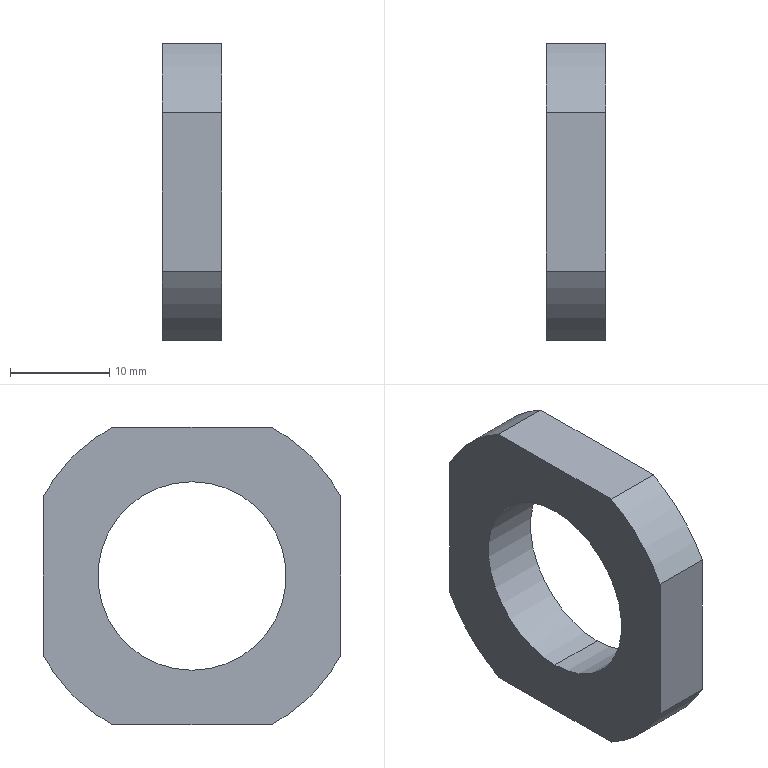Part | STEP file | PN_0005 nut | 1 solid | 12 faces | box 6 x 30 x 30 mm | volume 3228 mm3 | cylinder 6 | plane 6 | commonest cylinder face diameters 34 x4 19 x2
STEP:
#1=CARTESIAN_POINT('',(0.,0.,0.));
#2=DIRECTION('',(0.,0.,1.));
#3=DIRECTION('',(1.,0.,0.));
#4=AXIS2_PLACEMENT_3D('',#1,#2,#3);
#5=CARTESIAN_POINT('',(0.,0.,9.5));
#6=VERTEX_POINT('',#5);
#7=CARTESIAN_POINT('',(-6.,0.,9.5));
#8=VERTEX_POINT('',#7);
#9=CARTESIAN_POINT('',(0.,0.,9.5));
#10=DIRECTION('',(-1.,0.,0.));
#11=VECTOR('',#10,1.);
#12=LINE('',#9,#11);
#13=CARTESIAN_POINT('',(0.,0.,0.));
#14=DIRECTION('',(-1.,0.,0.));
#15=DIRECTION('',(0.,0.,1.));
#16=AXIS2_PLACEMENT_3D('',#13,#14,#15);
#17=CYLINDRICAL_SURFACE('',#16,9.5);
#18=CARTESIAN_POINT('',(6.283,0.));
#19=DIRECTION('',(0.,1.));
#20=VECTOR('',#19,1.);
#21=LINE('',#18,#20);
#22=(GEOMETRIC_REPRESENTATION_CONTEXT(2)PARAMETRIC_REPRESENTATION_CONTEXT()REPRESENTATION_CONTEXT('',''));
#23=DEFINITIONAL_REPRESENTATION('',(#21),#22);
#24=PCURVE('',#17,#23);
#25=CARTESIAN_POINT('',(0.,0.,0.));
#26=DIRECTION('',(-1.,0.,0.));
#27=DIRECTION('',(0.,0.,1.));
#28=AXIS2_PLACEMENT_3D('',#25,#26,#27);
#29=CYLINDRICAL_SURFACE('',#28,9.5);
#30=CARTESIAN_POINT('',(0.,0.));
#31=DIRECTION('',(0.,1.));
#32=VECTOR('',#31,1.);
#33=LINE('',#30,#32);
#34=(GEOMETRIC_REPRESENTATION_CONTEXT(2)PARAMETRIC_REPRESENTATION_CONTEXT()REPRESENTATION_CONTEXT('',''));
#35=DEFINITIONAL_REPRESENTATION('',(#33),#34);
#36=PCURVE('',#29,#35);
#37=SURFACE_CURVE('',#12,(#24,#36),.PCURVE_S1.);
#38=EDGE_CURVE('',#6,#8,#37,.T.);
#39=ORIENTED_EDGE('',*,*,#38,.T.);
#40=CARTESIAN_POINT('',(-6.,0.,-9.5));
#41=VERTEX_POINT('',#40);
#42=CARTESIAN_POINT('',(-6.,0.,0.));
#43=DIRECTION('',(1.,0.,0.));
#44=DIRECTION('',(0.,0.,-1.));
#45=AXIS2_PLACEMENT_3D('',#42,#43,#44);
#46=CIRCLE('',#45,9.5);
#47=CARTESIAN_POINT('',(9.425,6.));
#48=DIRECTION('',(-1.,0.));
#49=VECTOR('',#48,1.);
#50=LINE('',#47,#49);
#51=(GEOMETRIC_REPRESENTATION_CONTEXT(2)PARAMETRIC_REPRESENTATION_CONTEXT()REPRESENTATION_CONTEXT('',''));
#52=DEFINITIONAL_REPRESENTATION('',(#50),#51);
#53=PCURVE('',#17,#52);
#54=CARTESIAN_POINT('',(-6.,17.,0.));
#55=DIRECTION('',(-1.,0.,0.));
#56=DIRECTION('',(0.,0.,1.));
#57=AXIS2_PLACEMENT_3D('',#54,#55,#56);
#58=PLANE('',#57);
#59=CARTESIAN_POINT('',(-9.5,-17.));
#60=CARTESIAN_POINT('',(-9.5,-0.5455));
#61=CARTESIAN_POINT('',(4.75,-8.773));
#62=CARTESIAN_POINT('',(19.,-17.));
#63=CARTESIAN_POINT('',(4.75,-25.227));
#64=CARTESIAN_POINT('',(-9.5,-33.454));
#65=CARTESIAN_POINT('',(-9.5,-17.));
#66=(BOUNDED_CURVE()B_SPLINE_CURVE(2,(#59,#60,#61,#62,#63,#64,#65),.UNSPECIFIED.,.T.,.F.)B_SPLINE_CURVE_WITH_KNOTS((1,2,2,2,2,1),(-2.094,0.,2.094,4.189,6.283,8.378),.UNSPECIFIED.)CURVE()GEOMETRIC_REPRESENTATION_ITEM()RATIONAL_B_SPLINE_CURVE((1.,0.5,1.,0.5,1.,0.5,1.))REPRESENTATION_ITEM(''));
#67=(GEOMETRIC_REPRESENTATION_CONTEXT(2)PARAMETRIC_REPRESENTATION_CONTEXT()REPRESENTATION_CONTEXT('',''));
#68=DEFINITIONAL_REPRESENTATION('',(#66),#67);
#69=PCURVE('',#58,#68);
#70=SURFACE_CURVE('',#46,(#53,#69),.PCURVE_S1.);
#71=EDGE_CURVE('',#8,#41,#70,.T.);
#72=ORIENTED_EDGE('',*,*,#71,.T.);
#73=CARTESIAN_POINT('',(0.,0.,-9.5));
#74=VERTEX_POINT('',#73);
#75=CARTESIAN_POINT('',(0.,0.,-9.5));
#76=DIRECTION('',(-1.,0.,0.));
#77=VECTOR('',#76,1.);
#78=LINE('',#75,#77);
#79=CARTESIAN_POINT('',(3.142,0.));
#80=DIRECTION('',(0.,1.));
#81=VECTOR('',#80,1.);
#82=LINE('',#79,#81);
#83=(GEOMETRIC_REPRESENTATION_CONTEXT(2)PARAMETRIC_REPRESENTATION_CONTEXT()REPRESENTATION_CONTEXT('',''));
#84=DEFINITIONAL_REPRESENTATION('',(#82),#83);
#85=PCURVE('',#17,#84);
#86=CARTESIAN_POINT('',(3.142,0.));
#87=DIRECTION('',(0.,1.));
#88=VECTOR('',#87,1.);
#89=LINE('',#86,#88);
#90=(GEOMETRIC_REPRESENTATION_CONTEXT(2)PARAMETRIC_REPRESENTATION_CONTEXT()REPRESENTATION_CONTEXT('',''));
#91=DEFINITIONAL_REPRESENTATION('',(#89),#90);
#92=PCURVE('',#29,#91);
#93=SURFACE_CURVE('',#78,(#85,#92),.PCURVE_S1.);
#94=EDGE_CURVE('',#74,#41,#93,.T.);
#95=ORIENTED_EDGE('',*,*,#94,.F.);
#96=CARTESIAN_POINT('',(0.,0.,0.));
#97=DIRECTION('',(1.,0.,0.));
#98=DIRECTION('',(0.,0.,-1.));
#99=AXIS2_PLACEMENT_3D('',#96,#97,#98);
#100=CIRCLE('',#99,9.5);
#101=CARTESIAN_POINT('',(9.425,0.));
#102=DIRECTION('',(-1.,0.));
#103=VECTOR('',#102,1.);
#104=LINE('',#101,#103);
#105=(GEOMETRIC_REPRESENTATION_CONTEXT(2)PARAMETRIC_REPRESENTATION_CONTEXT()REPRESENTATION_CONTEXT('',''));
#106=DEFINITIONAL_REPRESENTATION('',(#104),#105);
#107=PCURVE('',#17,#106);
#108=CARTESIAN_POINT('',(0.,0.,0.));
#109=DIRECTION('',(1.,0.,0.));
#110=DIRECTION('',(0.,0.,-1.));
#111=AXIS2_PLACEMENT_3D('',#108,#109,#110);
#112=PLANE('',#111);
#113=CARTESIAN_POINT('',(0.,0.));
#114=DIRECTION('',(1.,0.));
#115=AXIS2_PLACEMENT_2D('',#113,#114);
#116=CIRCLE('',#115,9.5);
#117=(GEOMETRIC_REPRESENTATION_CONTEXT(2)PARAMETRIC_REPRESENTATION_CONTEXT()REPRESENTATION_CONTEXT('',''));
#118=DEFINITIONAL_REPRESENTATION('',(#116),#117);
#119=PCURVE('',#112,#118);
#120=SURFACE_CURVE('',#100,(#107,#119),.PCURVE_S1.);
#121=EDGE_CURVE('',#6,#74,#120,.T.);
#122=ORIENTED_EDGE('',*,*,#121,.F.);
#123=EDGE_LOOP('',(#39,#72,#95,#122));
#124=FACE_BOUND('',#123,.F.);
#125=ADVANCED_FACE('',(#124),#17,.F.);
#126=CARTESIAN_POINT('',(0.,8.,15.));
#127=VERTEX_POINT('',#126);
#128=CARTESIAN_POINT('',(-6.,8.,15.));
#129=VERTEX_POINT('',#128);
#130=CARTESIAN_POINT('',(0.,8.,15.));
#131=DIRECTION('',(-1.,0.,0.));
#132=VECTOR('',#131,1.);
#133=LINE('',#130,#132);
#134=CARTESIAN_POINT('',(0.,0.,0.));
#135=DIRECTION('',(1.,0.,0.));
#136=DIRECTION('',(0.,0.,-1.));
#137=AXIS2_PLACEMENT_3D('',#134,#135,#136);
#138=CYLINDRICAL_SURFACE('',#137,17.);
#139=CARTESIAN_POINT('',(2.652,0.));
#140=DIRECTION('',(0.,-1.));
#141=VECTOR('',#140,1.);
#142=LINE('',#139,#141);
#143=(GEOMETRIC_REPRESENTATION_CONTEXT(2)PARAMETRIC_REPRESENTATION_CONTEXT()REPRESENTATION_CONTEXT('',''));
#144=DEFINITIONAL_REPRESENTATION('',(#142),#143);
#145=PCURVE('',#138,#144);
#146=CARTESIAN_POINT('',(0.,17.205,15.));
#147=DIRECTION('',(0.,0.,-1.));
#148=DIRECTION('',(0.,1.,0.));
#149=AXIS2_PLACEMENT_3D('',#146,#147,#148);
#150=PLANE('',#149);
#151=CARTESIAN_POINT('',(-9.205,0.));
#152=DIRECTION('',(0.,-1.));
#153=VECTOR('',#152,1.);
#154=LINE('',#151,#153);
#155=(GEOMETRIC_REPRESENTATION_CONTEXT(2)PARAMETRIC_REPRESENTATION_CONTEXT()REPRESENTATION_CONTEXT('',''));
#156=DEFINITIONAL_REPRESENTATION('',(#154),#155);
#157=PCURVE('',#150,#156);
#158=SURFACE_CURVE('',#133,(#145,#157),.PCURVE_S1.);
#159=EDGE_CURVE('',#127,#129,#158,.T.);
#160=ORIENTED_EDGE('',*,*,#159,.F.);
#161=CARTESIAN_POINT('',(0.,15.,8.));
#162=VERTEX_POINT('',#161);
#163=CARTESIAN_POINT('',(0.,0.,0.));
#164=DIRECTION('',(1.,0.,0.));
#165=DIRECTION('',(0.,0.,-1.));
#166=AXIS2_PLACEMENT_3D('',#163,#164,#165);
#167=CIRCLE('',#166,17.);
#168=CARTESIAN_POINT('',(0.,0.));
#169=DIRECTION('',(1.,0.));
#170=VECTOR('',#169,1.);
#171=LINE('',#168,#170);
#172=(GEOMETRIC_REPRESENTATION_CONTEXT(2)PARAMETRIC_REPRESENTATION_CONTEXT()REPRESENTATION_CONTEXT('',''));
#173=DEFINITIONAL_REPRESENTATION('',(#171),#172);
#174=PCURVE('',#138,#173);
#175=CARTESIAN_POINT('',(0.,0.));
#176=DIRECTION('',(1.,0.));
#177=AXIS2_PLACEMENT_2D('',#175,#176);
#178=CIRCLE('',#177,17.);
#179=(GEOMETRIC_REPRESENTATION_CONTEXT(2)PARAMETRIC_REPRESENTATION_CONTEXT()REPRESENTATION_CONTEXT('',''));
#180=DEFINITIONAL_REPRESENTATION('',(#178),#179);
#181=PCURVE('',#112,#180);
#182=SURFACE_CURVE('',#167,(#174,#181),.PCURVE_S1.);
#183=EDGE_CURVE('',#162,#127,#182,.T.);
#184=ORIENTED_EDGE('',*,*,#183,.F.);
#185=CARTESIAN_POINT('',(-6.,15.,8.));
#186=VERTEX_POINT('',#185);
#187=CARTESIAN_POINT('',(0.,15.,8.));
#188=DIRECTION('',(1.,0.,0.));
#189=VECTOR('',#188,1.);
#190=LINE('',#187,#189);
#191=CARTESIAN_POINT('',(2.061,0.));
#192=DIRECTION('',(0.,1.));
#193=VECTOR('',#192,1.);
#194=LINE('',#191,#193);
#195=(GEOMETRIC_REPRESENTATION_CONTEXT(2)PARAMETRIC_REPRESENTATION_CONTEXT()REPRESENTATION_CONTEXT('',''));
#196=DEFINITIONAL_REPRESENTATION('',(#194),#195);
#197=PCURVE('',#138,#196);
#198=CARTESIAN_POINT('',(0.,15.,-20.296));
#199=DIRECTION('',(0.,-1.,0.));
#200=DIRECTION('',(0.,0.,-1.));
#201=AXIS2_PLACEMENT_3D('',#198,#199,#200);
#202=PLANE('',#201);
#203=CARTESIAN_POINT('',(-28.296,0.));
#204=DIRECTION('',(0.,1.));
#205=VECTOR('',#204,1.);
#206=LINE('',#203,#205);
#207=(GEOMETRIC_REPRESENTATION_CONTEXT(2)PARAMETRIC_REPRESENTATION_CONTEXT()REPRESENTATION_CONTEXT('',''));
#208=DEFINITIONAL_REPRESENTATION('',(#206),#207);
#209=PCURVE('',#202,#208);
#210=SURFACE_CURVE('',#190,(#197,#209),.PCURVE_S1.);
#211=EDGE_CURVE('',#186,#162,#210,.T.);
#212=ORIENTED_EDGE('',*,*,#211,.F.);
#213=CARTESIAN_POINT('',(-6.,0.,0.));
#214=DIRECTION('',(1.,0.,0.));
#215=DIRECTION('',(0.,0.,-1.));
#216=AXIS2_PLACEMENT_3D('',#213,#214,#215);
#217=CIRCLE('',#216,17.);
#218=CARTESIAN_POINT('',(0.,-6.));
#219=DIRECTION('',(1.,0.));
#220=VECTOR('',#219,1.);
#221=LINE('',#218,#220);
#222=(GEOMETRIC_REPRESENTATION_CONTEXT(2)PARAMETRIC_REPRESENTATION_CONTEXT()REPRESENTATION_CONTEXT('',''));
#223=DEFINITIONAL_REPRESENTATION('',(#221),#222);
#224=PCURVE('',#138,#223);
#225=CARTESIAN_POINT('',(-17.,-17.));
#226=CARTESIAN_POINT('',(-17.,12.445));
#227=CARTESIAN_POINT('',(8.5,-2.278));
#228=CARTESIAN_POINT('',(34.,-17.));
#229=CARTESIAN_POINT('',(8.5,-31.722));
#230=CARTESIAN_POINT('',(-17.,-46.445));
#231=CARTESIAN_POINT('',(-17.,-17.));
#232=(BOUNDED_CURVE()B_SPLINE_CURVE(2,(#225,#226,#227,#228,#229,#230,#231),.UNSPECIFIED.,.T.,.F.)B_SPLINE_CURVE_WITH_KNOTS((1,2,2,2,2,1),(-2.094,0.,2.094,4.189,6.283,8.378),.UNSPECIFIED.)CURVE()GEOMETRIC_REPRESENTATION_ITEM()RATIONAL_B_SPLINE_CURVE((1.,0.5,1.,0.5,1.,0.5,1.))REPRESENTATION_ITEM(''));
#233=(GEOMETRIC_REPRESENTATION_CONTEXT(2)PARAMETRIC_REPRESENTATION_CONTEXT()REPRESENTATION_CONTEXT('',''));
#234=DEFINITIONAL_REPRESENTATION('',(#232),#233);
#235=PCURVE('',#58,#234);
#236=SURFACE_CURVE('',#217,(#224,#235),.PCURVE_S1.);
#237=EDGE_CURVE('',#186,#129,#236,.T.);
#238=ORIENTED_EDGE('',*,*,#237,.T.);
#239=EDGE_LOOP('',(#160,#184,#212,#238));
#240=FACE_BOUND('',#239,.T.);
#241=ADVANCED_FACE('',(#240),#138,.T.);
#242=CARTESIAN_POINT('',(0.,-8.,-15.));
#243=VERTEX_POINT('',#242);
#244=CARTESIAN_POINT('',(-6.,-8.,-15.));
#245=VERTEX_POINT('',#244);
#246=CARTESIAN_POINT('',(0.,-8.,-15.));
#247=DIRECTION('',(-1.,0.,0.));
#248=VECTOR('',#247,1.);
#249=LINE('',#246,#248);
#250=CARTESIAN_POINT('',(0.,0.,0.));
#251=DIRECTION('',(1.,0.,0.));
#252=DIRECTION('',(0.,0.,-1.));
#253=AXIS2_PLACEMENT_3D('',#250,#251,#252);
#254=CYLINDRICAL_SURFACE('',#253,17.);
#255=CARTESIAN_POINT('',(5.793,0.));
#256=DIRECTION('',(0.,-1.));
#257=VECTOR('',#256,1.);
#258=LINE('',#255,#257);
#259=(GEOMETRIC_REPRESENTATION_CONTEXT(2)PARAMETRIC_REPRESENTATION_CONTEXT()REPRESENTATION_CONTEXT('',''));
#260=DEFINITIONAL_REPRESENTATION('',(#258),#259);
#261=PCURVE('',#254,#260);
#262=CARTESIAN_POINT('',(0.,17.205,-15.));
#263=DIRECTION('',(0.,0.,1.));
#264=DIRECTION('',(0.,-1.,0.));
#265=AXIS2_PLACEMENT_3D('',#262,#263,#264);
#266=PLANE('',#265);
#267=CARTESIAN_POINT('',(25.205,0.));
#268=DIRECTION('',(0.,-1.));
#269=VECTOR('',#268,1.);
#270=LINE('',#267,#269);
#271=(GEOMETRIC_REPRESENTATION_CONTEXT(2)PARAMETRIC_REPRESENTATION_CONTEXT()REPRESENTATION_CONTEXT('',''));
#272=DEFINITIONAL_REPRESENTATION('',(#270),#271);
#273=PCURVE('',#266,#272);
#274=SURFACE_CURVE('',#249,(#261,#273),.PCURVE_S1.);
#275=EDGE_CURVE('',#243,#245,#274,.T.);
#276=ORIENTED_EDGE('',*,*,#275,.F.);
#277=CARTESIAN_POINT('',(0.,-15.,-8.));
#278=VERTEX_POINT('',#277);
#279=CARTESIAN_POINT('',(0.,0.,0.));
#280=DIRECTION('',(1.,0.,0.));
#281=DIRECTION('',(0.,0.,-1.));
#282=AXIS2_PLACEMENT_3D('',#279,#280,#281);
#283=CIRCLE('',#282,17.);
#284=CARTESIAN_POINT('',(0.,0.));
#285=DIRECTION('',(1.,0.));
#286=VECTOR('',#285,1.);
#287=LINE('',#284,#286);
#288=(GEOMETRIC_REPRESENTATION_CONTEXT(2)PARAMETRIC_REPRESENTATION_CONTEXT()REPRESENTATION_CONTEXT('',''));
#289=DEFINITIONAL_REPRESENTATION('',(#287),#288);
#290=PCURVE('',#254,#289);
#291=CARTESIAN_POINT('',(0.,0.));
#292=DIRECTION('',(1.,0.));
#293=AXIS2_PLACEMENT_2D('',#291,#292);
#294=CIRCLE('',#293,17.);
#295=(GEOMETRIC_REPRESENTATION_CONTEXT(2)PARAMETRIC_REPRESENTATION_CONTEXT()REPRESENTATION_CONTEXT('',''));
#296=DEFINITIONAL_REPRESENTATION('',(#294),#295);
#297=PCURVE('',#112,#296);
#298=SURFACE_CURVE('',#283,(#290,#297),.PCURVE_S1.);
#299=EDGE_CURVE('',#278,#243,#298,.T.);
#300=ORIENTED_EDGE('',*,*,#299,.F.);
#301=CARTESIAN_POINT('',(-6.,-15.,-8.));
#302=VERTEX_POINT('',#301);
#303=CARTESIAN_POINT('',(0.,-15.,-8.));
#304=DIRECTION('',(1.,0.,0.));
#305=VECTOR('',#304,1.);
#306=LINE('',#303,#305);
#307=CARTESIAN_POINT('',(5.202,0.));
#308=DIRECTION('',(0.,1.));
#309=VECTOR('',#308,1.);
#310=LINE('',#307,#309);
#311=(GEOMETRIC_REPRESENTATION_CONTEXT(2)PARAMETRIC_REPRESENTATION_CONTEXT()REPRESENTATION_CONTEXT('',''));
#312=DEFINITIONAL_REPRESENTATION('',(#310),#311);
#313=PCURVE('',#254,#312);
#314=CARTESIAN_POINT('',(0.,-15.,-20.296));
#315=DIRECTION('',(0.,1.,0.));
#316=DIRECTION('',(0.,0.,1.));
#317=AXIS2_PLACEMENT_3D('',#314,#315,#316);
#318=PLANE('',#317);
#319=CARTESIAN_POINT('',(12.296,0.));
#320=DIRECTION('',(0.,1.));
#321=VECTOR('',#320,1.);
#322=LINE('',#319,#321);
#323=(GEOMETRIC_REPRESENTATION_CONTEXT(2)PARAMETRIC_REPRESENTATION_CONTEXT()REPRESENTATION_CONTEXT('',''));
#324=DEFINITIONAL_REPRESENTATION('',(#322),#323);
#325=PCURVE('',#318,#324);
#326=SURFACE_CURVE('',#306,(#313,#325),.PCURVE_S1.);
#327=EDGE_CURVE('',#302,#278,#326,.T.);
#328=ORIENTED_EDGE('',*,*,#327,.F.);
#329=CARTESIAN_POINT('',(-6.,0.,0.));
#330=DIRECTION('',(1.,0.,0.));
#331=DIRECTION('',(0.,0.,-1.));
#332=AXIS2_PLACEMENT_3D('',#329,#330,#331);
#333=CIRCLE('',#332,17.);
#334=CARTESIAN_POINT('',(0.,-6.));
#335=DIRECTION('',(1.,0.));
#336=VECTOR('',#335,1.);
#337=LINE('',#334,#336);
#338=(GEOMETRIC_REPRESENTATION_CONTEXT(2)PARAMETRIC_REPRESENTATION_CONTEXT()REPRESENTATION_CONTEXT('',''));
#339=DEFINITIONAL_REPRESENTATION('',(#337),#338);
#340=PCURVE('',#254,#339);
#341=CARTESIAN_POINT('',(-17.,-17.));
#342=CARTESIAN_POINT('',(-17.,12.445));
#343=CARTESIAN_POINT('',(8.5,-2.278));
#344=CARTESIAN_POINT('',(34.,-17.));
#345=CARTESIAN_POINT('',(8.5,-31.722));
#346=CARTESIAN_POINT('',(-17.,-46.445));
#347=CARTESIAN_POINT('',(-17.,-17.));
#348=(BOUNDED_CURVE()B_SPLINE_CURVE(2,(#341,#342,#343,#344,#345,#346,#347),.UNSPECIFIED.,.T.,.F.)B_SPLINE_CURVE_WITH_KNOTS((1,2,2,2,2,1),(-2.094,0.,2.094,4.189,6.283,8.378),.UNSPECIFIED.)CURVE()GEOMETRIC_REPRESENTATION_ITEM()RATIONAL_B_SPLINE_CURVE((1.,0.5,1.,0.5,1.,0.5,1.))REPRESENTATION_ITEM(''));
#349=(GEOMETRIC_REPRESENTATION_CONTEXT(2)PARAMETRIC_REPRESENTATION_CONTEXT()REPRESENTATION_CONTEXT('',''));
#350=DEFINITIONAL_REPRESENTATION('',(#348),#349);
#351=PCURVE('',#58,#350);
#352=SURFACE_CURVE('',#333,(#340,#351),.PCURVE_S1.);
#353=EDGE_CURVE('',#302,#245,#352,.T.);
#354=ORIENTED_EDGE('',*,*,#353,.T.);
#355=EDGE_LOOP('',(#276,#300,#328,#354));
#356=FACE_BOUND('',#355,.T.);
#357=ADVANCED_FACE('',(#356),#254,.T.);
#358=CARTESIAN_POINT('',(-6.,-8.,15.));
#359=VERTEX_POINT('',#358);
#360=CARTESIAN_POINT('',(0.,-8.,15.));
#361=VERTEX_POINT('',#360);
#362=CARTESIAN_POINT('',(0.,-8.,15.));
#363=DIRECTION('',(1.,0.,0.));
#364=VECTOR('',#363,1.);
#365=LINE('',#362,#364);
#366=CARTESIAN_POINT('',(0.,0.,0.));
#367=DIRECTION('',(1.,0.,0.));
#368=DIRECTION('',(0.,0.,-1.));
#369=AXIS2_PLACEMENT_3D('',#366,#367,#368);
#370=CYLINDRICAL_SURFACE('',#369,17.);
#371=CARTESIAN_POINT('',(3.632,0.));
#372=DIRECTION('',(0.,1.));
#373=VECTOR('',#372,1.);
#374=LINE('',#371,#373);
#375=(GEOMETRIC_REPRESENTATION_CONTEXT(2)PARAMETRIC_REPRESENTATION_CONTEXT()REPRESENTATION_CONTEXT('',''));
#376=DEFINITIONAL_REPRESENTATION('',(#374),#375);
#377=PCURVE('',#370,#376);
#378=CARTESIAN_POINT('',(-25.205,0.));
#379=DIRECTION('',(0.,1.));
#380=VECTOR('',#379,1.);
#381=LINE('',#378,#380);
#382=(GEOMETRIC_REPRESENTATION_CONTEXT(2)PARAMETRIC_REPRESENTATION_CONTEXT()REPRESENTATION_CONTEXT('',''));
#383=DEFINITIONAL_REPRESENTATION('',(#381),#382);
#384=PCURVE('',#150,#383);
#385=SURFACE_CURVE('',#365,(#377,#384),.PCURVE_S1.);
#386=EDGE_CURVE('',#359,#361,#385,.T.);
#387=ORIENTED_EDGE('',*,*,#386,.F.);
#388=CARTESIAN_POINT('',(-6.,-15.,8.));
#389=VERTEX_POINT('',#388);
#390=CARTESIAN_POINT('',(-6.,0.,0.));
#391=DIRECTION('',(1.,0.,0.));
#392=DIRECTION('',(0.,0.,-1.));
#393=AXIS2_PLACEMENT_3D('',#390,#391,#392);
#394=CIRCLE('',#393,17.);
#395=CARTESIAN_POINT('',(0.,-6.));
#396=DIRECTION('',(1.,0.));
#397=VECTOR('',#396,1.);
#398=LINE('',#395,#397);
#399=(GEOMETRIC_REPRESENTATION_CONTEXT(2)PARAMETRIC_REPRESENTATION_CONTEXT()REPRESENTATION_CONTEXT('',''));
#400=DEFINITIONAL_REPRESENTATION('',(#398),#399);
#401=PCURVE('',#370,#400);
#402=CARTESIAN_POINT('',(-17.,-17.));
#403=CARTESIAN_POINT('',(-17.,12.445));
#404=CARTESIAN_POINT('',(8.5,-2.278));
#405=CARTESIAN_POINT('',(34.,-17.));
#406=CARTESIAN_POINT('',(8.5,-31.722));
#407=CARTESIAN_POINT('',(-17.,-46.445));
#408=CARTESIAN_POINT('',(-17.,-17.));
#409=(BOUNDED_CURVE()B_SPLINE_CURVE(2,(#402,#403,#404,#405,#406,#407,#408),.UNSPECIFIED.,.T.,.F.)B_SPLINE_CURVE_WITH_KNOTS((1,2,2,2,2,1),(-2.094,0.,2.094,4.189,6.283,8.378),.UNSPECIFIED.)CURVE()GEOMETRIC_REPRESENTATION_ITEM()RATIONAL_B_SPLINE_CURVE((1.,0.5,1.,0.5,1.,0.5,1.))REPRESENTATION_ITEM(''));
#410=(GEOMETRIC_REPRESENTATION_CONTEXT(2)PARAMETRIC_REPRESENTATION_CONTEXT()REPRESENTATION_CONTEXT('',''));
#411=DEFINITIONAL_REPRESENTATION('',(#409),#410);
#412=PCURVE('',#58,#411);
#413=SURFACE_CURVE('',#394,(#401,#412),.PCURVE_S1.);
#414=EDGE_CURVE('',#359,#389,#413,.T.);
#415=ORIENTED_EDGE('',*,*,#414,.T.);
#416=CARTESIAN_POINT('',(0.,-15.,8.));
#417=VERTEX_POINT('',#416);
#418=CARTESIAN_POINT('',(0.,-15.,8.));
#419=DIRECTION('',(-1.,0.,0.));
#420=VECTOR('',#419,1.);
#421=LINE('',#418,#420);
#422=CARTESIAN_POINT('',(4.222,0.));
#423=DIRECTION('',(0.,-1.));
#424=VECTOR('',#423,1.);
#425=LINE('',#422,#424);
#426=(GEOMETRIC_REPRESENTATION_CONTEXT(2)PARAMETRIC_REPRESENTATION_CONTEXT()REPRESENTATION_CONTEXT('',''));
#427=DEFINITIONAL_REPRESENTATION('',(#425),#426);
#428=PCURVE('',#370,#427);
#429=CARTESIAN_POINT('',(28.296,0.));
#430=DIRECTION('',(0.,-1.));
#431=VECTOR('',#430,1.);
#432=LINE('',#429,#431);
#433=(GEOMETRIC_REPRESENTATION_CONTEXT(2)PARAMETRIC_REPRESENTATION_CONTEXT()REPRESENTATION_CONTEXT('',''));
#434=DEFINITIONAL_REPRESENTATION('',(#432),#433);
#435=PCURVE('',#318,#434);
#436=SURFACE_CURVE('',#421,(#428,#435),.PCURVE_S1.);
#437=EDGE_CURVE('',#417,#389,#436,.T.);
#438=ORIENTED_EDGE('',*,*,#437,.F.);
#439=CARTESIAN_POINT('',(0.,0.,0.));
#440=DIRECTION('',(1.,0.,0.));
#441=DIRECTION('',(0.,0.,-1.));
#442=AXIS2_PLACEMENT_3D('',#439,#440,#441);
#443=CIRCLE('',#442,17.);
#444=CARTESIAN_POINT('',(0.,0.));
#445=DIRECTION('',(1.,0.));
#446=VECTOR('',#445,1.);
#447=LINE('',#444,#446);
#448=(GEOMETRIC_REPRESENTATION_CONTEXT(2)PARAMETRIC_REPRESENTATION_CONTEXT()REPRESENTATION_CONTEXT('',''));
#449=DEFINITIONAL_REPRESENTATION('',(#447),#448);
#450=PCURVE('',#370,#449);
#451=CARTESIAN_POINT('',(0.,0.));
#452=DIRECTION('',(1.,0.));
#453=AXIS2_PLACEMENT_2D('',#451,#452);
#454=CIRCLE('',#453,17.);
#455=(GEOMETRIC_REPRESENTATION_CONTEXT(2)PARAMETRIC_REPRESENTATION_CONTEXT()REPRESENTATION_CONTEXT('',''));
#456=DEFINITIONAL_REPRESENTATION('',(#454),#455);
#457=PCURVE('',#112,#456);
#458=SURFACE_CURVE('',#443,(#450,#457),.PCURVE_S1.);
#459=EDGE_CURVE('',#361,#417,#458,.T.);
#460=ORIENTED_EDGE('',*,*,#459,.F.);
#461=EDGE_LOOP('',(#387,#415,#438,#460));
#462=FACE_BOUND('',#461,.T.);
#463=ADVANCED_FACE('',(#462),#370,.T.);
#464=CARTESIAN_POINT('',(0.,17.205,15.));
#465=DIRECTION('',(0.,-1.,0.));
#466=VECTOR('',#465,1.);
#467=LINE('',#464,#466);
#468=CARTESIAN_POINT('',(-15.,17.205));
#469=DIRECTION('',(0.,-1.));
#470=VECTOR('',#469,1.);
#471=LINE('',#468,#470);
#472=(GEOMETRIC_REPRESENTATION_CONTEXT(2)PARAMETRIC_REPRESENTATION_CONTEXT()REPRESENTATION_CONTEXT('',''));
#473=DEFINITIONAL_REPRESENTATION('',(#471),#472);
#474=PCURVE('',#112,#473);
#475=CARTESIAN_POINT('',(0.,0.));
#476=DIRECTION('',(-1.,0.));
#477=VECTOR('',#476,1.);
#478=LINE('',#475,#477);
#479=(GEOMETRIC_REPRESENTATION_CONTEXT(2)PARAMETRIC_REPRESENTATION_CONTEXT()REPRESENTATION_CONTEXT('',''));
#480=DEFINITIONAL_REPRESENTATION('',(#478),#479);
#481=PCURVE('',#150,#480);
#482=SURFACE_CURVE('',#467,(#474,#481),.PCURVE_S1.);
#483=EDGE_CURVE('',#127,#361,#482,.T.);
#484=ORIENTED_EDGE('',*,*,#483,.T.);
#485=ORIENTED_EDGE('',*,*,#459,.T.);
#486=CARTESIAN_POINT('',(0.,-15.,-20.296));
#487=DIRECTION('',(0.,0.,-1.));
#488=VECTOR('',#487,1.);
#489=LINE('',#486,#488);
#490=CARTESIAN_POINT('',(20.296,-15.));
#491=DIRECTION('',(1.,0.));
#492=VECTOR('',#491,1.);
#493=LINE('',#490,#492);
#494=(GEOMETRIC_REPRESENTATION_CONTEXT(2)PARAMETRIC_REPRESENTATION_CONTEXT()REPRESENTATION_CONTEXT('',''));
#495=DEFINITIONAL_REPRESENTATION('',(#493),#494);
#496=PCURVE('',#112,#495);
#497=CARTESIAN_POINT('',(0.,0.));
#498=DIRECTION('',(-1.,0.));
#499=VECTOR('',#498,1.);
#500=LINE('',#497,#499);
#501=(GEOMETRIC_REPRESENTATION_CONTEXT(2)PARAMETRIC_REPRESENTATION_CONTEXT()REPRESENTATION_CONTEXT('',''));
#502=DEFINITIONAL_REPRESENTATION('',(#500),#501);
#503=PCURVE('',#318,#502);
#504=SURFACE_CURVE('',#489,(#496,#503),.PCURVE_S1.);
#505=EDGE_CURVE('',#417,#278,#504,.T.);
#506=ORIENTED_EDGE('',*,*,#505,.T.);
#507=ORIENTED_EDGE('',*,*,#299,.T.);
#508=CARTESIAN_POINT('',(0.,8.,-15.));
#509=VERTEX_POINT('',#508);
#510=CARTESIAN_POINT('',(0.,17.205,-15.));
#511=DIRECTION('',(0.,1.,0.));
#512=VECTOR('',#511,1.);
#513=LINE('',#510,#512);
#514=CARTESIAN_POINT('',(15.,17.205));
#515=DIRECTION('',(0.,1.));
#516=VECTOR('',#515,1.);
#517=LINE('',#514,#516);
#518=(GEOMETRIC_REPRESENTATION_CONTEXT(2)PARAMETRIC_REPRESENTATION_CONTEXT()REPRESENTATION_CONTEXT('',''));
#519=DEFINITIONAL_REPRESENTATION('',(#517),#518);
#520=PCURVE('',#112,#519);
#521=CARTESIAN_POINT('',(0.,0.));
#522=DIRECTION('',(-1.,0.));
#523=VECTOR('',#522,1.);
#524=LINE('',#521,#523);
#525=(GEOMETRIC_REPRESENTATION_CONTEXT(2)PARAMETRIC_REPRESENTATION_CONTEXT()REPRESENTATION_CONTEXT('',''));
#526=DEFINITIONAL_REPRESENTATION('',(#524),#525);
#527=PCURVE('',#266,#526);
#528=SURFACE_CURVE('',#513,(#520,#527),.PCURVE_S1.);
#529=EDGE_CURVE('',#243,#509,#528,.T.);
#530=ORIENTED_EDGE('',*,*,#529,.T.);
#531=CARTESIAN_POINT('',(0.,15.,-8.));
#532=VERTEX_POINT('',#531);
#533=CARTESIAN_POINT('',(0.,0.,0.));
#534=DIRECTION('',(1.,0.,0.));
#535=DIRECTION('',(0.,0.,-1.));
#536=AXIS2_PLACEMENT_3D('',#533,#534,#535);
#537=CIRCLE('',#536,17.);
#538=CARTESIAN_POINT('',(0.,0.));
#539=DIRECTION('',(1.,0.));
#540=AXIS2_PLACEMENT_2D('',#538,#539);
#541=CIRCLE('',#540,17.);
#542=(GEOMETRIC_REPRESENTATION_CONTEXT(2)PARAMETRIC_REPRESENTATION_CONTEXT()REPRESENTATION_CONTEXT('',''));
#543=DEFINITIONAL_REPRESENTATION('',(#541),#542);
#544=PCURVE('',#112,#543);
#545=CARTESIAN_POINT('',(0.,0.,0.));
#546=DIRECTION('',(1.,0.,0.));
#547=DIRECTION('',(0.,0.,-1.));
#548=AXIS2_PLACEMENT_3D('',#545,#546,#547);
#549=CYLINDRICAL_SURFACE('',#548,17.);
#550=CARTESIAN_POINT('',(0.,0.));
#551=DIRECTION('',(1.,0.));
#552=VECTOR('',#551,1.);
#553=LINE('',#550,#552);
#554=(GEOMETRIC_REPRESENTATION_CONTEXT(2)PARAMETRIC_REPRESENTATION_CONTEXT()REPRESENTATION_CONTEXT('',''));
#555=DEFINITIONAL_REPRESENTATION('',(#553),#554);
#556=PCURVE('',#549,#555);
#557=SURFACE_CURVE('',#537,(#544,#556),.PCURVE_S1.);
#558=EDGE_CURVE('',#509,#532,#557,.T.);
#559=ORIENTED_EDGE('',*,*,#558,.T.);
#560=CARTESIAN_POINT('',(0.,15.,-20.296));
#561=DIRECTION('',(0.,0.,1.));
#562=VECTOR('',#561,1.);
#563=LINE('',#560,#562);
#564=CARTESIAN_POINT('',(20.296,15.));
#565=DIRECTION('',(-1.,0.));
#566=VECTOR('',#565,1.);
#567=LINE('',#564,#566);
#568=(GEOMETRIC_REPRESENTATION_CONTEXT(2)PARAMETRIC_REPRESENTATION_CONTEXT()REPRESENTATION_CONTEXT('',''));
#569=DEFINITIONAL_REPRESENTATION('',(#567),#568);
#570=PCURVE('',#112,#569);
#571=CARTESIAN_POINT('',(0.,0.));
#572=DIRECTION('',(-1.,0.));
#573=VECTOR('',#572,1.);
#574=LINE('',#571,#573);
#575=(GEOMETRIC_REPRESENTATION_CONTEXT(2)PARAMETRIC_REPRESENTATION_CONTEXT()REPRESENTATION_CONTEXT('',''));
#576=DEFINITIONAL_REPRESENTATION('',(#574),#575);
#577=PCURVE('',#202,#576);
#578=SURFACE_CURVE('',#563,(#570,#577),.PCURVE_S1.);
#579=EDGE_CURVE('',#532,#162,#578,.T.);
#580=ORIENTED_EDGE('',*,*,#579,.T.);
#581=ORIENTED_EDGE('',*,*,#183,.T.);
#582=EDGE_LOOP('',(#484,#485,#506,#507,#530,#559,#580,#581));
#583=FACE_BOUND('',#582,.T.);
#584=ORIENTED_EDGE('',*,*,#121,.F.);
#585=CARTESIAN_POINT('',(0.,0.,0.));
#586=DIRECTION('',(1.,0.,0.));
#587=DIRECTION('',(0.,0.,-1.));
#588=AXIS2_PLACEMENT_3D('',#585,#586,#587);
#589=CIRCLE('',#588,9.5);
#590=CARTESIAN_POINT('',(0.,0.));
#591=DIRECTION('',(1.,0.));
#592=AXIS2_PLACEMENT_2D('',#590,#591);
#593=CIRCLE('',#592,9.5);
#594=(GEOMETRIC_REPRESENTATION_CONTEXT(2)PARAMETRIC_REPRESENTATION_CONTEXT()REPRESENTATION_CONTEXT('',''));
#595=DEFINITIONAL_REPRESENTATION('',(#593),#594);
#596=PCURVE('',#112,#595);
#597=CARTESIAN_POINT('',(3.142,0.));
#598=DIRECTION('',(-1.,0.));
#599=VECTOR('',#598,1.);
#600=LINE('',#597,#599);
#601=(GEOMETRIC_REPRESENTATION_CONTEXT(2)PARAMETRIC_REPRESENTATION_CONTEXT()REPRESENTATION_CONTEXT('',''));
#602=DEFINITIONAL_REPRESENTATION('',(#600),#601);
#603=PCURVE('',#29,#602);
#604=SURFACE_CURVE('',#589,(#596,#603),.PCURVE_S1.);
#605=EDGE_CURVE('',#74,#6,#604,.T.);
#606=ORIENTED_EDGE('',*,*,#605,.F.);
#607=EDGE_LOOP('',(#584,#606));
#608=FACE_BOUND('',#607,.T.);
#609=ADVANCED_FACE('',(#583,#608),#112,.T.);
#610=CARTESIAN_POINT('',(-6.,17.,15.));
#611=DIRECTION('',(0.,-1.,0.));
#612=VECTOR('',#611,1.);
#613=LINE('',#610,#612);
#614=CARTESIAN_POINT('',(15.,0.));
#615=DIRECTION('',(0.,-1.));
#616=VECTOR('',#615,1.);
#617=LINE('',#614,#616);
#618=(GEOMETRIC_REPRESENTATION_CONTEXT(2)PARAMETRIC_REPRESENTATION_CONTEXT()REPRESENTATION_CONTEXT('',''));
#619=DEFINITIONAL_REPRESENTATION('',(#617),#618);
#620=PCURVE('',#58,#619);
#621=CARTESIAN_POINT('',(-0.2052,-6.));
#622=DIRECTION('',(-1.,0.));
#623=VECTOR('',#622,1.);
#624=LINE('',#621,#623);
#625=(GEOMETRIC_REPRESENTATION_CONTEXT(2)PARAMETRIC_REPRESENTATION_CONTEXT()REPRESENTATION_CONTEXT('',''));
#626=DEFINITIONAL_REPRESENTATION('',(#624),#625);
#627=PCURVE('',#150,#626);
#628=SURFACE_CURVE('',#613,(#620,#627),.PCURVE_S1.);
#629=EDGE_CURVE('',#129,#359,#628,.T.);
#630=ORIENTED_EDGE('',*,*,#629,.F.);
#631=ORIENTED_EDGE('',*,*,#237,.F.);
#632=CARTESIAN_POINT('',(-6.,15.,-8.));
#633=VERTEX_POINT('',#632);
#634=CARTESIAN_POINT('',(-6.,15.,-20.296));
#635=DIRECTION('',(0.,0.,1.));
#636=VECTOR('',#635,1.);
#637=LINE('',#634,#636);
#638=CARTESIAN_POINT('',(-20.296,-2.));
#639=DIRECTION('',(1.,0.));
#640=VECTOR('',#639,1.);
#641=LINE('',#638,#640);
#642=(GEOMETRIC_REPRESENTATION_CONTEXT(2)PARAMETRIC_REPRESENTATION_CONTEXT()REPRESENTATION_CONTEXT('',''));
#643=DEFINITIONAL_REPRESENTATION('',(#641),#642);
#644=PCURVE('',#58,#643);
#645=CARTESIAN_POINT('',(0.,-6.));
#646=DIRECTION('',(-1.,0.));
#647=VECTOR('',#646,1.);
#648=LINE('',#645,#647);
#649=(GEOMETRIC_REPRESENTATION_CONTEXT(2)PARAMETRIC_REPRESENTATION_CONTEXT()REPRESENTATION_CONTEXT('',''));
#650=DEFINITIONAL_REPRESENTATION('',(#648),#649);
#651=PCURVE('',#202,#650);
#652=SURFACE_CURVE('',#637,(#644,#651),.PCURVE_S1.);
#653=EDGE_CURVE('',#633,#186,#652,.T.);
#654=ORIENTED_EDGE('',*,*,#653,.F.);
#655=CARTESIAN_POINT('',(-6.,8.,-15.));
#656=VERTEX_POINT('',#655);
#657=CARTESIAN_POINT('',(-6.,0.,0.));
#658=DIRECTION('',(1.,0.,0.));
#659=DIRECTION('',(0.,0.,-1.));
#660=AXIS2_PLACEMENT_3D('',#657,#658,#659);
#661=CIRCLE('',#660,17.);
#662=CARTESIAN_POINT('',(-17.,-17.));
#663=CARTESIAN_POINT('',(-17.,12.445));
#664=CARTESIAN_POINT('',(8.5,-2.278));
#665=CARTESIAN_POINT('',(34.,-17.));
#666=CARTESIAN_POINT('',(8.5,-31.722));
#667=CARTESIAN_POINT('',(-17.,-46.445));
#668=CARTESIAN_POINT('',(-17.,-17.));
#669=(BOUNDED_CURVE()B_SPLINE_CURVE(2,(#662,#663,#664,#665,#666,#667,#668),.UNSPECIFIED.,.T.,.F.)B_SPLINE_CURVE_WITH_KNOTS((1,2,2,2,2,1),(-2.094,0.,2.094,4.189,6.283,8.378),.UNSPECIFIED.)CURVE()GEOMETRIC_REPRESENTATION_ITEM()RATIONAL_B_SPLINE_CURVE((1.,0.5,1.,0.5,1.,0.5,1.))REPRESENTATION_ITEM(''));
#670=(GEOMETRIC_REPRESENTATION_CONTEXT(2)PARAMETRIC_REPRESENTATION_CONTEXT()REPRESENTATION_CONTEXT('',''));
#671=DEFINITIONAL_REPRESENTATION('',(#669),#670);
#672=PCURVE('',#58,#671);
#673=CARTESIAN_POINT('',(0.,-6.));
#674=DIRECTION('',(1.,0.));
#675=VECTOR('',#674,1.);
#676=LINE('',#673,#675);
#677=(GEOMETRIC_REPRESENTATION_CONTEXT(2)PARAMETRIC_REPRESENTATION_CONTEXT()REPRESENTATION_CONTEXT('',''));
#678=DEFINITIONAL_REPRESENTATION('',(#676),#677);
#679=PCURVE('',#549,#678);
#680=SURFACE_CURVE('',#661,(#672,#679),.PCURVE_S1.);
#681=EDGE_CURVE('',#656,#633,#680,.T.);
#682=ORIENTED_EDGE('',*,*,#681,.F.);
#683=CARTESIAN_POINT('',(-6.,17.205,-15.));
#684=DIRECTION('',(0.,1.,0.));
#685=VECTOR('',#684,1.);
#686=LINE('',#683,#685);
#687=CARTESIAN_POINT('',(-15.,0.2052));
#688=DIRECTION('',(0.,1.));
#689=VECTOR('',#688,1.);
#690=LINE('',#687,#689);
#691=(GEOMETRIC_REPRESENTATION_CONTEXT(2)PARAMETRIC_REPRESENTATION_CONTEXT()REPRESENTATION_CONTEXT('',''));
#692=DEFINITIONAL_REPRESENTATION('',(#690),#691);
#693=PCURVE('',#58,#692);
#694=CARTESIAN_POINT('',(0.,-6.));
#695=DIRECTION('',(-1.,0.));
#696=VECTOR('',#695,1.);
#697=LINE('',#694,#696);
#698=(GEOMETRIC_REPRESENTATION_CONTEXT(2)PARAMETRIC_REPRESENTATION_CONTEXT()REPRESENTATION_CONTEXT('',''));
#699=DEFINITIONAL_REPRESENTATION('',(#697),#698);
#700=PCURVE('',#266,#699);
#701=SURFACE_CURVE('',#686,(#693,#700),.PCURVE_S1.);
#702=EDGE_CURVE('',#245,#656,#701,.T.);
#703=ORIENTED_EDGE('',*,*,#702,.F.);
#704=ORIENTED_EDGE('',*,*,#353,.F.);
#705=CARTESIAN_POINT('',(-6.,-15.,-20.296));
#706=DIRECTION('',(0.,0.,-1.));
#707=VECTOR('',#706,1.);
#708=LINE('',#705,#707);
#709=CARTESIAN_POINT('',(-20.296,-32.));
#710=DIRECTION('',(-1.,0.));
#711=VECTOR('',#710,1.);
#712=LINE('',#709,#711);
#713=(GEOMETRIC_REPRESENTATION_CONTEXT(2)PARAMETRIC_REPRESENTATION_CONTEXT()REPRESENTATION_CONTEXT('',''));
#714=DEFINITIONAL_REPRESENTATION('',(#712),#713);
#715=PCURVE('',#58,#714);
#716=CARTESIAN_POINT('',(0.,-6.));
#717=DIRECTION('',(-1.,0.));
#718=VECTOR('',#717,1.);
#719=LINE('',#716,#718);
#720=(GEOMETRIC_REPRESENTATION_CONTEXT(2)PARAMETRIC_REPRESENTATION_CONTEXT()REPRESENTATION_CONTEXT('',''));
#721=DEFINITIONAL_REPRESENTATION('',(#719),#720);
#722=PCURVE('',#318,#721);
#723=SURFACE_CURVE('',#708,(#715,#722),.PCURVE_S1.);
#724=EDGE_CURVE('',#389,#302,#723,.T.);
#725=ORIENTED_EDGE('',*,*,#724,.F.);
#726=ORIENTED_EDGE('',*,*,#414,.F.);
#727=EDGE_LOOP('',(#630,#631,#654,#682,#703,#704,#725,#726));
#728=FACE_BOUND('',#727,.T.);
#729=ORIENTED_EDGE('',*,*,#71,.T.);
#730=CARTESIAN_POINT('',(-6.,0.,0.));
#731=DIRECTION('',(1.,0.,0.));
#732=DIRECTION('',(0.,0.,-1.));
#733=AXIS2_PLACEMENT_3D('',#730,#731,#732);
#734=CIRCLE('',#733,9.5);
#735=CARTESIAN_POINT('',(-9.5,-17.));
#736=CARTESIAN_POINT('',(-9.5,-0.5455));
#737=CARTESIAN_POINT('',(4.75,-8.773));
#738=CARTESIAN_POINT('',(19.,-17.));
#739=CARTESIAN_POINT('',(4.75,-25.227));
#740=CARTESIAN_POINT('',(-9.5,-33.454));
#741=CARTESIAN_POINT('',(-9.5,-17.));
#742=(BOUNDED_CURVE()B_SPLINE_CURVE(2,(#735,#736,#737,#738,#739,#740,#741),.UNSPECIFIED.,.T.,.F.)B_SPLINE_CURVE_WITH_KNOTS((1,2,2,2,2,1),(-2.094,0.,2.094,4.189,6.283,8.378),.UNSPECIFIED.)CURVE()GEOMETRIC_REPRESENTATION_ITEM()RATIONAL_B_SPLINE_CURVE((1.,0.5,1.,0.5,1.,0.5,1.))REPRESENTATION_ITEM(''));
#743=(GEOMETRIC_REPRESENTATION_CONTEXT(2)PARAMETRIC_REPRESENTATION_CONTEXT()REPRESENTATION_CONTEXT('',''));
#744=DEFINITIONAL_REPRESENTATION('',(#742),#743);
#745=PCURVE('',#58,#744);
#746=CARTESIAN_POINT('',(3.142,6.));
#747=DIRECTION('',(-1.,0.));
#748=VECTOR('',#747,1.);
#749=LINE('',#746,#748);
#750=(GEOMETRIC_REPRESENTATION_CONTEXT(2)PARAMETRIC_REPRESENTATION_CONTEXT()REPRESENTATION_CONTEXT('',''));
#751=DEFINITIONAL_REPRESENTATION('',(#749),#750);
#752=PCURVE('',#29,#751);
#753=SURFACE_CURVE('',#734,(#745,#752),.PCURVE_S1.);
#754=EDGE_CURVE('',#41,#8,#753,.T.);
#755=ORIENTED_EDGE('',*,*,#754,.T.);
#756=EDGE_LOOP('',(#729,#755));
#757=FACE_BOUND('',#756,.T.);
#758=ADVANCED_FACE('',(#728,#757),#58,.T.);
#759=CARTESIAN_POINT('',(0.,8.,-15.));
#760=DIRECTION('',(1.,0.,0.));
#761=VECTOR('',#760,1.);
#762=LINE('',#759,#761);
#763=CARTESIAN_POINT('',(0.49,0.));
#764=DIRECTION('',(0.,1.));
#765=VECTOR('',#764,1.);
#766=LINE('',#763,#765);
#767=(GEOMETRIC_REPRESENTATION_CONTEXT(2)PARAMETRIC_REPRESENTATION_CONTEXT()REPRESENTATION_CONTEXT('',''));
#768=DEFINITIONAL_REPRESENTATION('',(#766),#767);
#769=PCURVE('',#549,#768);
#770=CARTESIAN_POINT('',(9.205,0.));
#771=DIRECTION('',(0.,1.));
#772=VECTOR('',#771,1.);
#773=LINE('',#770,#772);
#774=(GEOMETRIC_REPRESENTATION_CONTEXT(2)PARAMETRIC_REPRESENTATION_CONTEXT()REPRESENTATION_CONTEXT('',''));
#775=DEFINITIONAL_REPRESENTATION('',(#773),#774);
#776=PCURVE('',#266,#775);
#777=SURFACE_CURVE('',#762,(#769,#776),.PCURVE_S1.);
#778=EDGE_CURVE('',#656,#509,#777,.T.);
#779=ORIENTED_EDGE('',*,*,#778,.F.);
#780=ORIENTED_EDGE('',*,*,#681,.T.);
#781=CARTESIAN_POINT('',(0.,15.,-8.));
#782=DIRECTION('',(-1.,0.,0.));
#783=VECTOR('',#782,1.);
#784=LINE('',#781,#783);
#785=CARTESIAN_POINT('',(1.081,0.));
#786=DIRECTION('',(0.,-1.));
#787=VECTOR('',#786,1.);
#788=LINE('',#785,#787);
#789=(GEOMETRIC_REPRESENTATION_CONTEXT(2)PARAMETRIC_REPRESENTATION_CONTEXT()REPRESENTATION_CONTEXT('',''));
#790=DEFINITIONAL_REPRESENTATION('',(#788),#789);
#791=PCURVE('',#549,#790);
#792=CARTESIAN_POINT('',(-12.296,0.));
#793=DIRECTION('',(0.,-1.));
#794=VECTOR('',#793,1.);
#795=LINE('',#792,#794);
#796=(GEOMETRIC_REPRESENTATION_CONTEXT(2)PARAMETRIC_REPRESENTATION_CONTEXT()REPRESENTATION_CONTEXT('',''));
#797=DEFINITIONAL_REPRESENTATION('',(#795),#796);
#798=PCURVE('',#202,#797);
#799=SURFACE_CURVE('',#784,(#791,#798),.PCURVE_S1.);
#800=EDGE_CURVE('',#532,#633,#799,.T.);
#801=ORIENTED_EDGE('',*,*,#800,.F.);
#802=ORIENTED_EDGE('',*,*,#558,.F.);
#803=EDGE_LOOP('',(#779,#780,#801,#802));
#804=FACE_BOUND('',#803,.T.);
#805=ADVANCED_FACE('',(#804),#549,.T.);
#806=ORIENTED_EDGE('',*,*,#754,.T.);
#807=ORIENTED_EDGE('',*,*,#38,.F.);
#808=ORIENTED_EDGE('',*,*,#605,.F.);
#809=ORIENTED_EDGE('',*,*,#94,.T.);
#810=EDGE_LOOP('',(#806,#807,#808,#809));
#811=FACE_BOUND('',#810,.F.);
#812=ADVANCED_FACE('',(#811),#29,.F.);
#813=ORIENTED_EDGE('',*,*,#800,.T.);
#814=ORIENTED_EDGE('',*,*,#653,.T.);
#815=ORIENTED_EDGE('',*,*,#211,.T.);
#816=ORIENTED_EDGE('',*,*,#579,.F.);
#817=EDGE_LOOP('',(#813,#814,#815,#816));
#818=FACE_BOUND('',#817,.T.);
#819=ADVANCED_FACE('',(#818),#202,.F.);
#820=ORIENTED_EDGE('',*,*,#437,.T.);
#821=ORIENTED_EDGE('',*,*,#724,.T.);
#822=ORIENTED_EDGE('',*,*,#327,.T.);
#823=ORIENTED_EDGE('',*,*,#505,.F.);
#824=EDGE_LOOP('',(#820,#821,#822,#823));
#825=FACE_BOUND('',#824,.T.);
#826=ADVANCED_FACE('',(#825),#318,.F.);
#827=ORIENTED_EDGE('',*,*,#275,.T.);
#828=ORIENTED_EDGE('',*,*,#702,.T.);
#829=ORIENTED_EDGE('',*,*,#778,.T.);
#830=ORIENTED_EDGE('',*,*,#529,.F.);
#831=EDGE_LOOP('',(#827,#828,#829,#830));
#832=FACE_BOUND('',#831,.T.);
#833=ADVANCED_FACE('',(#832),#266,.F.);
#834=ORIENTED_EDGE('',*,*,#159,.T.);
#835=ORIENTED_EDGE('',*,*,#629,.T.);
#836=ORIENTED_EDGE('',*,*,#386,.T.);
#837=ORIENTED_EDGE('',*,*,#483,.F.);
#838=EDGE_LOOP('',(#834,#835,#836,#837));
#839=FACE_BOUND('',#838,.T.);
#840=ADVANCED_FACE('',(#839),#150,.F.);
#841=CLOSED_SHELL('',(#125,#241,#357,#463,#609,#758,#805,#812,#819,#826,#833,#840));
#842=MANIFOLD_SOLID_BREP('',#841);
#843=(LENGTH_UNIT()NAMED_UNIT(*)SI_UNIT(.MILLI.,.METRE.));
#844=UNCERTAINTY_MEASURE_WITH_UNIT(LENGTH_MEASURE(0.0000001),#843,'','');
#845=(NAMED_UNIT(*)PLANE_ANGLE_UNIT()SI_UNIT($,.RADIAN.));
#846=(NAMED_UNIT(*)SI_UNIT($,.STERADIAN.)SOLID_ANGLE_UNIT());
#847=(GEOMETRIC_REPRESENTATION_CONTEXT(3)GLOBAL_UNCERTAINTY_ASSIGNED_CONTEXT((#844))GLOBAL_UNIT_ASSIGNED_CONTEXT((#843,#845,#846))REPRESENTATION_CONTEXT('',''));
#848=ADVANCED_BREP_SHAPE_REPRESENTATION('',(#4,#842),#847);